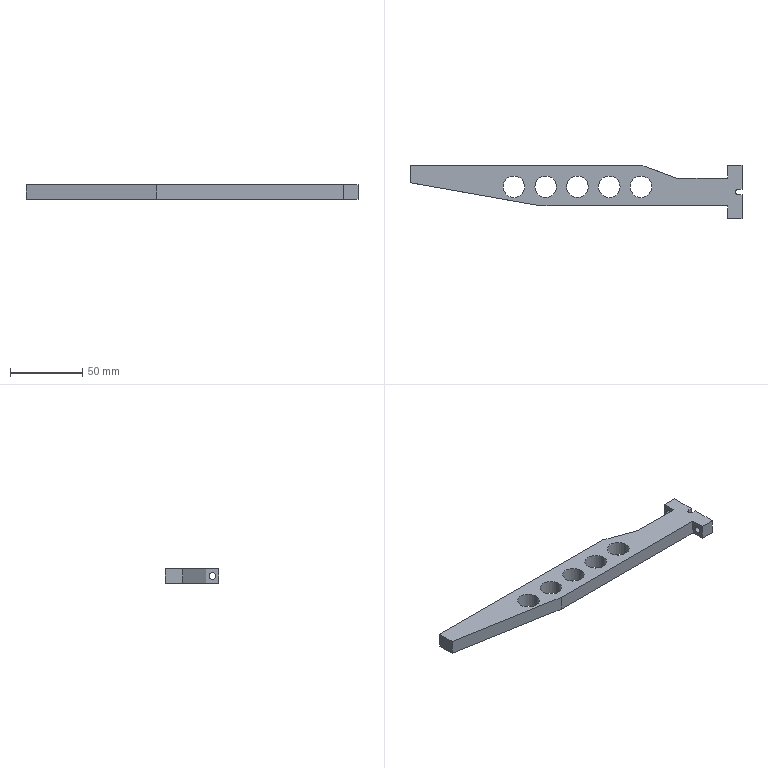CAM job | NX | 3-axis milling | part box 230 x 37.2 x 10 mm | stock box 236 x 43.2 x 11 mm
Tools:
number,name,description,diameter,corner_radius,flute_length,length,flutes
1,D50,Milling Tool-5 Parameters,50.0,0.0,50.0,75.0,2
3,D10,Milling Tool-5 Parameters,10.0,0.0,50.0,75.0,2
4,D10JING,Milling Tool-5 Parameters,10.0,0.0,50.0,75.0,2
2,D6A45,Milling Tool-5 Parameters,6.0,0.0,3.0,3.0,2
8,D6,Milling Tool-5 Parameters,6.0,0.0,50.0,75.0,2
13,D3,Milling Tool-5 Parameters,3.0,0.0,50.0,75.0,2
Operations:
program,operation,operation_type,tool,method,geometry_group,spindle_rpm,surface_speed,feed_per_tooth,feed_cut,feed_plunge,cut_length_mm,path_length_mm,cut_time_min,machine_time_min
1-233-40-12毛胚,FLOOR_WALL,VolumeBased25DMillingOperation,D50,METHOD,A,6500.0,1286.0,0.0962,1250.0,100.0,298.0,352.0,0.2384,0.2438
1-233-40-12毛胚,ADAPTIVE_MILLING,CavityMilling,D10,METHOD,A,7000.0,219.0,0.1571,2200.0,1000.0,8228.304,12398.433,3.765,4.182
1-233-40-12毛胚,HOLE_MILLING,CylinderMilling,D10,METHOD,A,7000.0,131.0,0.1071,1500.0,100.0,1104.091,1539.591,0.7361,0.7796
1-233-40-12毛胚,ZLEVEL_PROFILE_COPY_COPY_1_COPY_COPY_COPY_1,ZLevelMilling,D10JING,METHOD,A,7000.0,219.0,0.0714,1000.0,100.0,656.547,1496.671,0.6565,0.7406
1-233-40-12毛胚,ZLEVEL_PROFILE_COPY_COPY_1_COPY_COPY_COPY_1_COPY_COPY_1,ZLevelMilling,D6,METHOD,A,7000.0,131.0,0.1071,1500.0,100.0,402.659,1002.791,0.2684,0.3285
1-233-40-12毛胚,ZLEVEL_PROFILE_COPY_COPY_1_COPY_COPY_COPY_1_COPY_COPY_1_COPY,ZLevelMilling,D3,METHOD,A,7000.0,65.0,0.0857,1200.0,100.0,548.93,1158.947,0.4574,0.5184
1-233-40-12毛胚,ZLEVEL_PROFILE_COPY_COPY_1_COPY_COPY_COPY_1_COPY_COPY_1_COPY_COPY,ZLevelMilling,D3,METHOD,A,7000.0,131.0,0.0857,1200.0,100.0,531.324,739.933,0.4428,0.4636
1-233-40-12毛胚,ZLEVEL_PROFILE_COPY_1_COPY_COPY_COPY_COPY_2_COPY,ZLevelMilling,D6A45,METHOD,A,7000.0,131.0,0.0714,1000.0,1000.0,769.459,1451.278,0.7695,0.8376
1-233-40-12毛胚,刀补13,ZLevelMilling,D3,METHOD,A,7000.0,131.0,0.0607,850.0,100.0,65.729,145.864,0.0773,0.0853